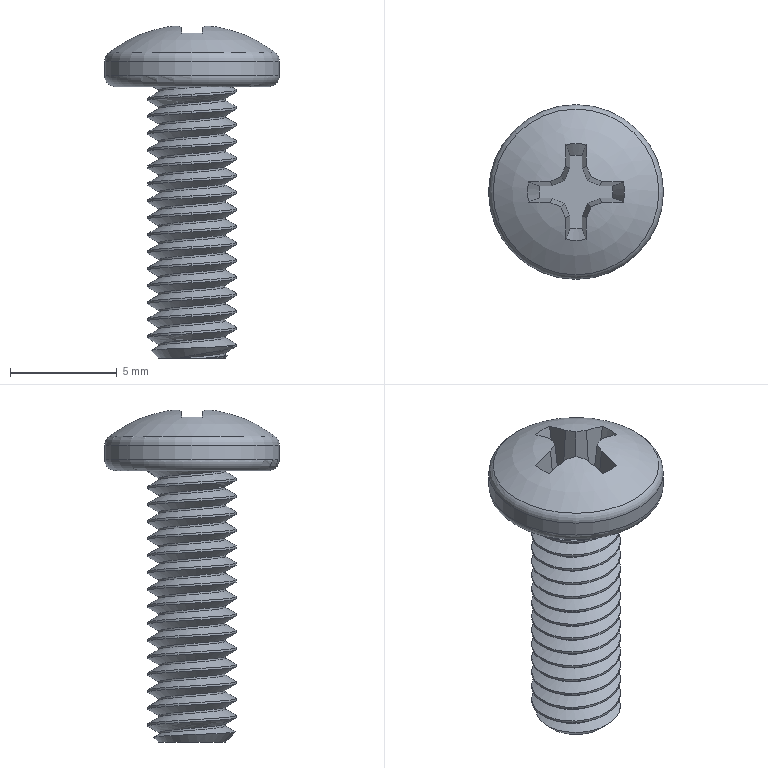Part | NX | features solid 2 | 1 solid | 64 faces | box 8.179 x 8.179 x 15.544 mm | volume 243.583 mm3 | cylinder 34 | plane 19 | cone 5 | spline 3 | torus 2 | sphere 1 | commonest cylinder face diameters 4.166 x32 3.134 x1 8.179 x1